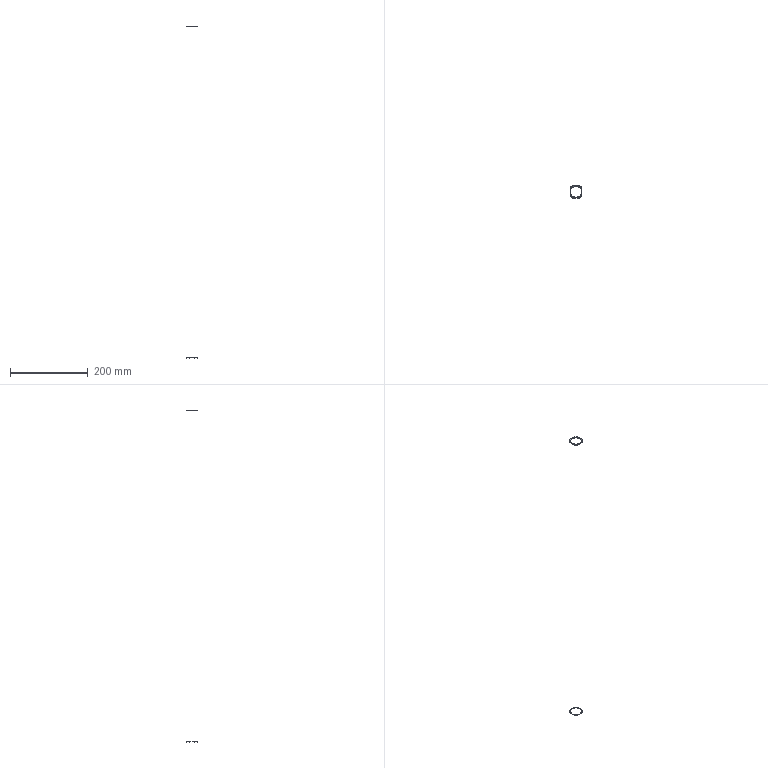Part | SolidWorks | features BaseBody 5 | 5 solids | 63 faces | box 30 x 30 x 855 mm | volume 282.424 mm3 | plane 25 | cylinder 24 | cone 14 | commonest cylinder face diameters 15 x16 9 x8